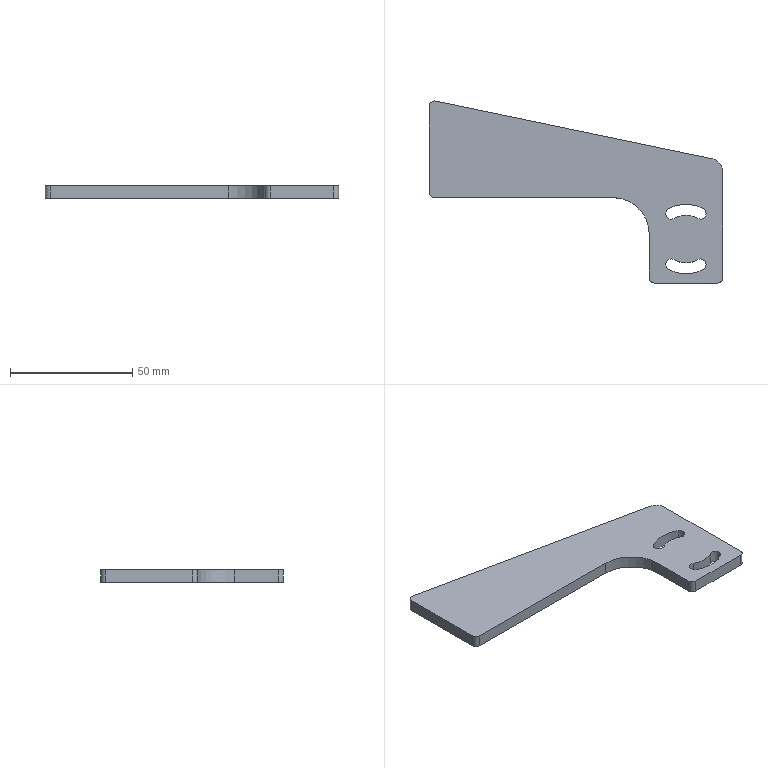Part | STEP file | Planar support stopper | 1 solid | 24 faces | box 120 x 74.54 x 5 mm | volume 21231 mm3 | cylinder 16 | plane 8 | commonest cylinder face diameters 4.5 x6 4 x4 19.5 x2 28.5 x2 10 x1 30 x1